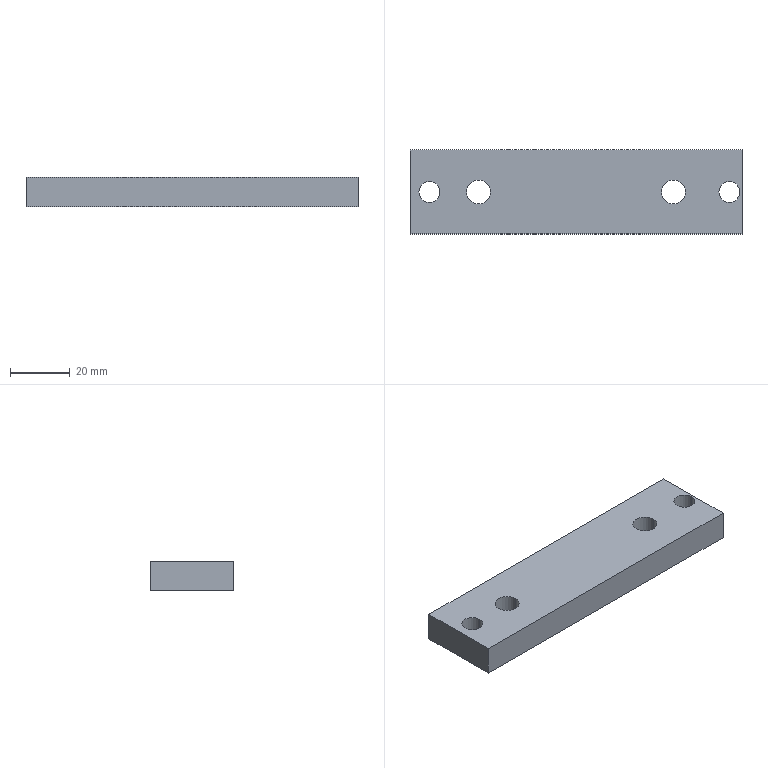Part | STEP file | 导柱Plate-2 | 1 solid | 14 faces | box 110.709 x 28 x 10 mm | volume 29224 mm3 | cylinder 8 | plane 6 | commonest cylinder face diameters 7 x4 8 x4
STEP:
#1=CARTESIAN_POINT('',(13.5,0.,10.));
#2=VERTEX_POINT('',#1);
#3=CARTESIAN_POINT('',(21.5,0.,10.));
#4=VERTEX_POINT('',#3);
#5=CARTESIAN_POINT('',(17.5,0.,10.));
#6=DIRECTION('',(0.,0.,1.));
#7=DIRECTION('',(1.,0.,0.));
#8=AXIS2_PLACEMENT_3D('',#5,#6,#7);
#9=CIRCLE('',#8,4.);
#10=EDGE_CURVE('',#2,#4,#9,.T.);
#11=ORIENTED_EDGE('',*,*,#10,.T.);
#12=CARTESIAN_POINT('',(21.5,0.,0.));
#13=VERTEX_POINT('',#12);
#14=CARTESIAN_POINT('',(21.5,0.,10.));
#15=DIRECTION('',(0.,0.,-1.));
#16=VECTOR('',#15,1000.);
#17=LINE('',#14,#16);
#18=EDGE_CURVE('',#4,#13,#17,.T.);
#19=ORIENTED_EDGE('',*,*,#18,.T.);
#20=CARTESIAN_POINT('',(13.5,0.,0.));
#21=VERTEX_POINT('',#20);
#22=CARTESIAN_POINT('',(17.5,0.,0.));
#23=DIRECTION('',(0.,0.,1.));
#24=DIRECTION('',(1.,0.,0.));
#25=AXIS2_PLACEMENT_3D('',#22,#23,#24);
#26=CIRCLE('',#25,4.);
#27=EDGE_CURVE('',#21,#13,#26,.T.);
#28=ORIENTED_EDGE('',*,*,#27,.F.);
#29=CARTESIAN_POINT('',(13.5,0.,10.));
#30=DIRECTION('',(0.,0.,-1.));
#31=VECTOR('',#30,1000.);
#32=LINE('',#29,#31);
#33=EDGE_CURVE('',#2,#21,#32,.T.);
#34=ORIENTED_EDGE('',*,*,#33,.F.);
#35=EDGE_LOOP('',(#11,#19,#28,#34));
#36=FACE_OUTER_BOUND('',#35,.T.);
#37=CARTESIAN_POINT('',(17.5,0.,10.));
#38=DIRECTION('',(0.,0.,-1.));
#39=DIRECTION('',(-1.,0.,0.));
#40=AXIS2_PLACEMENT_3D('',#37,#38,#39);
#41=CYLINDRICAL_SURFACE('',#40,4.);
#42=ADVANCED_FACE('',(#36),#41,.F.);
#43=CARTESIAN_POINT('',(78.5,0.,10.));
#44=VERTEX_POINT('',#43);
#45=CARTESIAN_POINT('',(86.5,0.,10.));
#46=VERTEX_POINT('',#45);
#47=CARTESIAN_POINT('',(82.5,0.,10.));
#48=DIRECTION('',(0.,0.,1.));
#49=DIRECTION('',(1.,0.,0.));
#50=AXIS2_PLACEMENT_3D('',#47,#48,#49);
#51=CIRCLE('',#50,4.);
#52=EDGE_CURVE('',#44,#46,#51,.T.);
#53=ORIENTED_EDGE('',*,*,#52,.T.);
#54=CARTESIAN_POINT('',(86.5,0.,0.));
#55=VERTEX_POINT('',#54);
#56=CARTESIAN_POINT('',(86.5,0.,10.));
#57=DIRECTION('',(0.,0.,-1.));
#58=VECTOR('',#57,1000.);
#59=LINE('',#56,#58);
#60=EDGE_CURVE('',#46,#55,#59,.T.);
#61=ORIENTED_EDGE('',*,*,#60,.T.);
#62=CARTESIAN_POINT('',(78.5,0.,0.));
#63=VERTEX_POINT('',#62);
#64=CARTESIAN_POINT('',(82.5,0.,0.));
#65=DIRECTION('',(0.,0.,1.));
#66=DIRECTION('',(1.,0.,0.));
#67=AXIS2_PLACEMENT_3D('',#64,#65,#66);
#68=CIRCLE('',#67,4.);
#69=EDGE_CURVE('',#63,#55,#68,.T.);
#70=ORIENTED_EDGE('',*,*,#69,.F.);
#71=CARTESIAN_POINT('',(78.5,0.,10.));
#72=DIRECTION('',(0.,0.,-1.));
#73=VECTOR('',#72,1000.);
#74=LINE('',#71,#73);
#75=EDGE_CURVE('',#44,#63,#74,.T.);
#76=ORIENTED_EDGE('',*,*,#75,.F.);
#77=EDGE_LOOP('',(#53,#61,#70,#76));
#78=FACE_OUTER_BOUND('',#77,.T.);
#79=CARTESIAN_POINT('',(82.5,0.,10.));
#80=DIRECTION('',(0.,0.,-1.));
#81=DIRECTION('',(-1.,0.,0.));
#82=AXIS2_PLACEMENT_3D('',#79,#80,#81);
#83=CYLINDRICAL_SURFACE('',#82,4.);
#84=ADVANCED_FACE('',(#78),#83,.F.);
#85=CARTESIAN_POINT('',(97.645,0.,10.));
#86=VERTEX_POINT('',#85);
#87=CARTESIAN_POINT('',(104.645,0.,10.));
#88=VERTEX_POINT('',#87);
#89=CARTESIAN_POINT('',(101.145,0.,10.));
#90=DIRECTION('',(0.,0.,1.));
#91=DIRECTION('',(1.,0.,0.));
#92=AXIS2_PLACEMENT_3D('',#89,#90,#91);
#93=CIRCLE('',#92,3.5);
#94=EDGE_CURVE('',#86,#88,#93,.T.);
#95=ORIENTED_EDGE('',*,*,#94,.T.);
#96=CARTESIAN_POINT('',(104.645,0.,0.));
#97=VERTEX_POINT('',#96);
#98=CARTESIAN_POINT('',(104.645,0.,10.));
#99=DIRECTION('',(0.,0.,-1.));
#100=VECTOR('',#99,1000.);
#101=LINE('',#98,#100);
#102=EDGE_CURVE('',#88,#97,#101,.T.);
#103=ORIENTED_EDGE('',*,*,#102,.T.);
#104=CARTESIAN_POINT('',(97.645,0.,0.));
#105=VERTEX_POINT('',#104);
#106=CARTESIAN_POINT('',(101.145,0.,0.));
#107=DIRECTION('',(0.,0.,1.));
#108=DIRECTION('',(1.,0.,0.));
#109=AXIS2_PLACEMENT_3D('',#106,#107,#108);
#110=CIRCLE('',#109,3.5);
#111=EDGE_CURVE('',#105,#97,#110,.T.);
#112=ORIENTED_EDGE('',*,*,#111,.F.);
#113=CARTESIAN_POINT('',(97.645,0.,10.));
#114=DIRECTION('',(0.,0.,-1.));
#115=VECTOR('',#114,1000.);
#116=LINE('',#113,#115);
#117=EDGE_CURVE('',#86,#105,#116,.T.);
#118=ORIENTED_EDGE('',*,*,#117,.F.);
#119=EDGE_LOOP('',(#95,#103,#112,#118));
#120=FACE_OUTER_BOUND('',#119,.T.);
#121=CARTESIAN_POINT('',(101.145,0.,10.));
#122=DIRECTION('',(0.,0.,-1.));
#123=DIRECTION('',(-1.,0.,0.));
#124=AXIS2_PLACEMENT_3D('',#121,#122,#123);
#125=CYLINDRICAL_SURFACE('',#124,3.5);
#126=ADVANCED_FACE('',(#120),#125,.F.);
#127=CARTESIAN_POINT('',(-2.355,0.,10.));
#128=VERTEX_POINT('',#127);
#129=CARTESIAN_POINT('',(4.645,0.,10.));
#130=VERTEX_POINT('',#129);
#131=CARTESIAN_POINT('',(1.145,0.,10.));
#132=DIRECTION('',(0.,0.,1.));
#133=DIRECTION('',(1.,0.,0.));
#134=AXIS2_PLACEMENT_3D('',#131,#132,#133);
#135=CIRCLE('',#134,3.5);
#136=EDGE_CURVE('',#128,#130,#135,.T.);
#137=ORIENTED_EDGE('',*,*,#136,.T.);
#138=CARTESIAN_POINT('',(4.645,0.,0.));
#139=VERTEX_POINT('',#138);
#140=CARTESIAN_POINT('',(4.645,0.,10.));
#141=DIRECTION('',(0.,0.,-1.));
#142=VECTOR('',#141,1000.);
#143=LINE('',#140,#142);
#144=EDGE_CURVE('',#130,#139,#143,.T.);
#145=ORIENTED_EDGE('',*,*,#144,.T.);
#146=CARTESIAN_POINT('',(-2.355,0.,0.));
#147=VERTEX_POINT('',#146);
#148=CARTESIAN_POINT('',(1.145,0.,0.));
#149=DIRECTION('',(0.,0.,1.));
#150=DIRECTION('',(1.,0.,0.));
#151=AXIS2_PLACEMENT_3D('',#148,#149,#150);
#152=CIRCLE('',#151,3.5);
#153=EDGE_CURVE('',#147,#139,#152,.T.);
#154=ORIENTED_EDGE('',*,*,#153,.F.);
#155=CARTESIAN_POINT('',(-2.355,0.,10.));
#156=DIRECTION('',(0.,0.,-1.));
#157=VECTOR('',#156,1000.);
#158=LINE('',#155,#157);
#159=EDGE_CURVE('',#128,#147,#158,.T.);
#160=ORIENTED_EDGE('',*,*,#159,.F.);
#161=EDGE_LOOP('',(#137,#145,#154,#160));
#162=FACE_OUTER_BOUND('',#161,.T.);
#163=CARTESIAN_POINT('',(1.145,0.,10.));
#164=DIRECTION('',(0.,0.,-1.));
#165=DIRECTION('',(-1.,0.,0.));
#166=AXIS2_PLACEMENT_3D('',#163,#164,#165);
#167=CYLINDRICAL_SURFACE('',#166,3.5);
#168=ADVANCED_FACE('',(#162),#167,.F.);
#169=ORIENTED_EDGE('',*,*,#52,.F.);
#170=CARTESIAN_POINT('',(82.5,0.,10.));
#171=DIRECTION('',(0.,0.,1.));
#172=DIRECTION('',(1.,0.,0.));
#173=AXIS2_PLACEMENT_3D('',#170,#171,#172);
#174=CIRCLE('',#173,4.);
#175=EDGE_CURVE('',#46,#44,#174,.T.);
#176=ORIENTED_EDGE('',*,*,#175,.F.);
#177=EDGE_LOOP('',(#169,#176));
#178=FACE_BOUND('',#177,.T.);
#179=ORIENTED_EDGE('',*,*,#136,.F.);
#180=CARTESIAN_POINT('',(1.145,0.,10.));
#181=DIRECTION('',(0.,0.,1.));
#182=DIRECTION('',(1.,0.,0.));
#183=AXIS2_PLACEMENT_3D('',#180,#181,#182);
#184=CIRCLE('',#183,3.5);
#185=EDGE_CURVE('',#130,#128,#184,.T.);
#186=ORIENTED_EDGE('',*,*,#185,.F.);
#187=EDGE_LOOP('',(#179,#186));
#188=FACE_BOUND('',#187,.T.);
#189=CARTESIAN_POINT('',(105.355,-14.,10.));
#190=VERTEX_POINT('',#189);
#191=CARTESIAN_POINT('',(105.355,14.,10.));
#192=VERTEX_POINT('',#191);
#193=CARTESIAN_POINT('',(105.355,-14.,10.));
#194=DIRECTION('',(0.,1.,0.));
#195=VECTOR('',#194,1000.);
#196=LINE('',#193,#195);
#197=EDGE_CURVE('',#190,#192,#196,.T.);
#198=ORIENTED_EDGE('',*,*,#197,.T.);
#199=CARTESIAN_POINT('',(-5.355,14.,10.));
#200=VERTEX_POINT('',#199);
#201=CARTESIAN_POINT('',(-5.355,14.,10.));
#202=DIRECTION('',(-1.,0.,0.));
#203=VECTOR('',#202,1000.);
#204=LINE('',#201,#203);
#205=EDGE_CURVE('',#192,#200,#204,.T.);
#206=ORIENTED_EDGE('',*,*,#205,.T.);
#207=CARTESIAN_POINT('',(-5.355,-14.,10.));
#208=VERTEX_POINT('',#207);
#209=CARTESIAN_POINT('',(-5.355,-14.,10.));
#210=DIRECTION('',(0.,-1.,0.));
#211=VECTOR('',#210,1000.);
#212=LINE('',#209,#211);
#213=EDGE_CURVE('',#200,#208,#212,.T.);
#214=ORIENTED_EDGE('',*,*,#213,.T.);
#215=CARTESIAN_POINT('',(-5.355,-14.,10.));
#216=DIRECTION('',(1.,0.,0.));
#217=VECTOR('',#216,1000.);
#218=LINE('',#215,#217);
#219=EDGE_CURVE('',#208,#190,#218,.T.);
#220=ORIENTED_EDGE('',*,*,#219,.T.);
#221=EDGE_LOOP('',(#198,#206,#214,#220));
#222=FACE_OUTER_BOUND('',#221,.T.);
#223=ORIENTED_EDGE('',*,*,#94,.F.);
#224=CARTESIAN_POINT('',(101.145,0.,10.));
#225=DIRECTION('',(0.,0.,1.));
#226=DIRECTION('',(1.,0.,0.));
#227=AXIS2_PLACEMENT_3D('',#224,#225,#226);
#228=CIRCLE('',#227,3.5);
#229=EDGE_CURVE('',#88,#86,#228,.T.);
#230=ORIENTED_EDGE('',*,*,#229,.F.);
#231=EDGE_LOOP('',(#223,#230));
#232=FACE_BOUND('',#231,.T.);
#233=ORIENTED_EDGE('',*,*,#10,.F.);
#234=CARTESIAN_POINT('',(17.5,0.,10.));
#235=DIRECTION('',(0.,0.,1.));
#236=DIRECTION('',(1.,0.,0.));
#237=AXIS2_PLACEMENT_3D('',#234,#235,#236);
#238=CIRCLE('',#237,4.);
#239=EDGE_CURVE('',#4,#2,#238,.T.);
#240=ORIENTED_EDGE('',*,*,#239,.F.);
#241=EDGE_LOOP('',(#233,#240));
#242=FACE_BOUND('',#241,.T.);
#243=CARTESIAN_POINT('',(105.355,14.,10.));
#244=DIRECTION('',(0.,0.,-1.));
#245=DIRECTION('',(-1.,0.,0.));
#246=AXIS2_PLACEMENT_3D('',#243,#244,#245);
#247=PLANE('',#246);
#248=ADVANCED_FACE('',(#178,#188,#222,#232,#242),#247,.F.);
#249=ORIENTED_EDGE('',*,*,#69,.T.);
#250=CARTESIAN_POINT('',(82.5,0.,0.));
#251=DIRECTION('',(0.,0.,1.));
#252=DIRECTION('',(1.,0.,0.));
#253=AXIS2_PLACEMENT_3D('',#250,#251,#252);
#254=CIRCLE('',#253,4.);
#255=EDGE_CURVE('',#55,#63,#254,.T.);
#256=ORIENTED_EDGE('',*,*,#255,.T.);
#257=EDGE_LOOP('',(#249,#256));
#258=FACE_BOUND('',#257,.T.);
#259=ORIENTED_EDGE('',*,*,#153,.T.);
#260=CARTESIAN_POINT('',(1.145,0.,0.));
#261=DIRECTION('',(0.,0.,1.));
#262=DIRECTION('',(1.,0.,0.));
#263=AXIS2_PLACEMENT_3D('',#260,#261,#262);
#264=CIRCLE('',#263,3.5);
#265=EDGE_CURVE('',#139,#147,#264,.T.);
#266=ORIENTED_EDGE('',*,*,#265,.T.);
#267=EDGE_LOOP('',(#259,#266));
#268=FACE_BOUND('',#267,.T.);
#269=CARTESIAN_POINT('',(105.355,-14.,0.));
#270=VERTEX_POINT('',#269);
#271=CARTESIAN_POINT('',(105.355,14.,0.));
#272=VERTEX_POINT('',#271);
#273=CARTESIAN_POINT('',(105.355,-14.,0.));
#274=DIRECTION('',(0.,1.,0.));
#275=VECTOR('',#274,1000.);
#276=LINE('',#273,#275);
#277=EDGE_CURVE('',#270,#272,#276,.T.);
#278=ORIENTED_EDGE('',*,*,#277,.F.);
#279=CARTESIAN_POINT('',(-5.355,-14.,0.));
#280=VERTEX_POINT('',#279);
#281=CARTESIAN_POINT('',(-5.355,-14.,0.));
#282=DIRECTION('',(1.,0.,0.));
#283=VECTOR('',#282,1000.);
#284=LINE('',#281,#283);
#285=EDGE_CURVE('',#280,#270,#284,.T.);
#286=ORIENTED_EDGE('',*,*,#285,.F.);
#287=CARTESIAN_POINT('',(-5.355,14.,0.));
#288=VERTEX_POINT('',#287);
#289=CARTESIAN_POINT('',(-5.355,-14.,0.));
#290=DIRECTION('',(0.,-1.,0.));
#291=VECTOR('',#290,1000.);
#292=LINE('',#289,#291);
#293=EDGE_CURVE('',#288,#280,#292,.T.);
#294=ORIENTED_EDGE('',*,*,#293,.F.);
#295=CARTESIAN_POINT('',(-5.355,14.,0.));
#296=DIRECTION('',(-1.,0.,0.));
#297=VECTOR('',#296,1000.);
#298=LINE('',#295,#297);
#299=EDGE_CURVE('',#272,#288,#298,.T.);
#300=ORIENTED_EDGE('',*,*,#299,.F.);
#301=EDGE_LOOP('',(#278,#286,#294,#300));
#302=FACE_OUTER_BOUND('',#301,.T.);
#303=ORIENTED_EDGE('',*,*,#111,.T.);
#304=CARTESIAN_POINT('',(101.145,0.,0.));
#305=DIRECTION('',(0.,0.,1.));
#306=DIRECTION('',(1.,0.,0.));
#307=AXIS2_PLACEMENT_3D('',#304,#305,#306);
#308=CIRCLE('',#307,3.5);
#309=EDGE_CURVE('',#97,#105,#308,.T.);
#310=ORIENTED_EDGE('',*,*,#309,.T.);
#311=EDGE_LOOP('',(#303,#310));
#312=FACE_BOUND('',#311,.T.);
#313=ORIENTED_EDGE('',*,*,#27,.T.);
#314=CARTESIAN_POINT('',(17.5,0.,0.));
#315=DIRECTION('',(0.,0.,1.));
#316=DIRECTION('',(1.,0.,0.));
#317=AXIS2_PLACEMENT_3D('',#314,#315,#316);
#318=CIRCLE('',#317,4.);
#319=EDGE_CURVE('',#13,#21,#318,.T.);
#320=ORIENTED_EDGE('',*,*,#319,.T.);
#321=EDGE_LOOP('',(#313,#320));
#322=FACE_BOUND('',#321,.T.);
#323=CARTESIAN_POINT('',(105.355,14.,0.));
#324=DIRECTION('',(0.,0.,-1.));
#325=DIRECTION('',(-1.,0.,0.));
#326=AXIS2_PLACEMENT_3D('',#323,#324,#325);
#327=PLANE('',#326);
#328=ADVANCED_FACE('',(#258,#268,#302,#312,#322),#327,.T.);
#329=ORIENTED_EDGE('',*,*,#277,.T.);
#330=CARTESIAN_POINT('',(105.355,14.,10.));
#331=DIRECTION('',(0.,0.,-1.));
#332=VECTOR('',#331,1000.);
#333=LINE('',#330,#332);
#334=EDGE_CURVE('',#192,#272,#333,.T.);
#335=ORIENTED_EDGE('',*,*,#334,.F.);
#336=ORIENTED_EDGE('',*,*,#197,.F.);
#337=CARTESIAN_POINT('',(105.355,-14.,10.));
#338=DIRECTION('',(0.,0.,-1.));
#339=VECTOR('',#338,1000.);
#340=LINE('',#337,#339);
#341=EDGE_CURVE('',#190,#270,#340,.T.);
#342=ORIENTED_EDGE('',*,*,#341,.T.);
#343=EDGE_LOOP('',(#329,#335,#336,#342));
#344=FACE_OUTER_BOUND('',#343,.T.);
#345=CARTESIAN_POINT('',(105.355,-14.,10.));
#346=DIRECTION('',(-1.,0.,0.));
#347=DIRECTION('',(0.,0.,1.));
#348=AXIS2_PLACEMENT_3D('',#345,#346,#347);
#349=PLANE('',#348);
#350=ADVANCED_FACE('',(#344),#349,.F.);
#351=ORIENTED_EDGE('',*,*,#299,.T.);
#352=CARTESIAN_POINT('',(-5.355,14.,10.));
#353=DIRECTION('',(0.,0.,-1.));
#354=VECTOR('',#353,1000.);
#355=LINE('',#352,#354);
#356=EDGE_CURVE('',#200,#288,#355,.T.);
#357=ORIENTED_EDGE('',*,*,#356,.F.);
#358=ORIENTED_EDGE('',*,*,#205,.F.);
#359=ORIENTED_EDGE('',*,*,#334,.T.);
#360=EDGE_LOOP('',(#351,#357,#358,#359));
#361=FACE_OUTER_BOUND('',#360,.T.);
#362=CARTESIAN_POINT('',(-5.355,14.,10.));
#363=DIRECTION('',(0.,-1.,0.));
#364=DIRECTION('',(0.,0.,-1.));
#365=AXIS2_PLACEMENT_3D('',#362,#363,#364);
#366=PLANE('',#365);
#367=ADVANCED_FACE('',(#361),#366,.F.);
#368=ORIENTED_EDGE('',*,*,#293,.T.);
#369=CARTESIAN_POINT('',(-5.355,-14.,10.));
#370=DIRECTION('',(0.,0.,-1.));
#371=VECTOR('',#370,1000.);
#372=LINE('',#369,#371);
#373=EDGE_CURVE('',#208,#280,#372,.T.);
#374=ORIENTED_EDGE('',*,*,#373,.F.);
#375=ORIENTED_EDGE('',*,*,#213,.F.);
#376=ORIENTED_EDGE('',*,*,#356,.T.);
#377=EDGE_LOOP('',(#368,#374,#375,#376));
#378=FACE_OUTER_BOUND('',#377,.T.);
#379=CARTESIAN_POINT('',(-5.355,-14.,10.));
#380=DIRECTION('',(1.,0.,0.));
#381=DIRECTION('',(0.,0.,-1.));
#382=AXIS2_PLACEMENT_3D('',#379,#380,#381);
#383=PLANE('',#382);
#384=ADVANCED_FACE('',(#378),#383,.F.);
#385=ORIENTED_EDGE('',*,*,#285,.T.);
#386=ORIENTED_EDGE('',*,*,#341,.F.);
#387=ORIENTED_EDGE('',*,*,#219,.F.);
#388=ORIENTED_EDGE('',*,*,#373,.T.);
#389=EDGE_LOOP('',(#385,#386,#387,#388));
#390=FACE_OUTER_BOUND('',#389,.T.);
#391=CARTESIAN_POINT('',(-5.355,-14.,10.));
#392=DIRECTION('',(0.,1.,0.));
#393=DIRECTION('',(0.,0.,1.));
#394=AXIS2_PLACEMENT_3D('',#391,#392,#393);
#395=PLANE('',#394);
#396=ADVANCED_FACE('',(#390),#395,.F.);
#397=ORIENTED_EDGE('',*,*,#144,.F.);
#398=ORIENTED_EDGE('',*,*,#185,.T.);
#399=ORIENTED_EDGE('',*,*,#159,.T.);
#400=ORIENTED_EDGE('',*,*,#265,.F.);
#401=EDGE_LOOP('',(#397,#398,#399,#400));
#402=FACE_OUTER_BOUND('',#401,.T.);
#403=CARTESIAN_POINT('',(1.145,0.,10.));
#404=DIRECTION('',(0.,0.,-1.));
#405=DIRECTION('',(-1.,0.,0.));
#406=AXIS2_PLACEMENT_3D('',#403,#404,#405);
#407=CYLINDRICAL_SURFACE('',#406,3.5);
#408=ADVANCED_FACE('',(#402),#407,.F.);
#409=ORIENTED_EDGE('',*,*,#102,.F.);
#410=ORIENTED_EDGE('',*,*,#229,.T.);
#411=ORIENTED_EDGE('',*,*,#117,.T.);
#412=ORIENTED_EDGE('',*,*,#309,.F.);
#413=EDGE_LOOP('',(#409,#410,#411,#412));
#414=FACE_OUTER_BOUND('',#413,.T.);
#415=CARTESIAN_POINT('',(101.145,0.,10.));
#416=DIRECTION('',(0.,0.,-1.));
#417=DIRECTION('',(-1.,0.,0.));
#418=AXIS2_PLACEMENT_3D('',#415,#416,#417);
#419=CYLINDRICAL_SURFACE('',#418,3.5);
#420=ADVANCED_FACE('',(#414),#419,.F.);
#421=ORIENTED_EDGE('',*,*,#60,.F.);
#422=ORIENTED_EDGE('',*,*,#175,.T.);
#423=ORIENTED_EDGE('',*,*,#75,.T.);
#424=ORIENTED_EDGE('',*,*,#255,.F.);
#425=EDGE_LOOP('',(#421,#422,#423,#424));
#426=FACE_OUTER_BOUND('',#425,.T.);
#427=CARTESIAN_POINT('',(82.5,0.,10.));
#428=DIRECTION('',(0.,0.,-1.));
#429=DIRECTION('',(-1.,0.,0.));
#430=AXIS2_PLACEMENT_3D('',#427,#428,#429);
#431=CYLINDRICAL_SURFACE('',#430,4.);
#432=ADVANCED_FACE('',(#426),#431,.F.);
#433=ORIENTED_EDGE('',*,*,#18,.F.);
#434=ORIENTED_EDGE('',*,*,#239,.T.);
#435=ORIENTED_EDGE('',*,*,#33,.T.);
#436=ORIENTED_EDGE('',*,*,#319,.F.);
#437=EDGE_LOOP('',(#433,#434,#435,#436));
#438=FACE_OUTER_BOUND('',#437,.T.);
#439=CARTESIAN_POINT('',(17.5,0.,10.));
#440=DIRECTION('',(0.,0.,-1.));
#441=DIRECTION('',(-1.,0.,0.));
#442=AXIS2_PLACEMENT_3D('',#439,#440,#441);
#443=CYLINDRICAL_SURFACE('',#442,4.);
#444=ADVANCED_FACE('',(#438),#443,.F.);
#445=CLOSED_SHELL('',(#42,#84,#126,#168,#248,#328,#350,#367,#384,#396,#408,#420,#432,#444));
#446=MANIFOLD_SOLID_BREP('',#445);
#447=CARTESIAN_POINT('',(0.,0.,0.));
#448=DIRECTION('',(0.,0.,1.));
#449=DIRECTION('',(1.,0.,0.));
#450=AXIS2_PLACEMENT_3D('',#447,#448,#449);
#451=(LENGTH_UNIT()NAMED_UNIT(*)SI_UNIT(.MILLI.,.METRE.));
#452=UNCERTAINTY_MEASURE_WITH_UNIT(LENGTH_MEASURE(0.00001),#451,'','');
#453=(NAMED_UNIT(*)PLANE_ANGLE_UNIT()SI_UNIT($,.RADIAN.));
#454=(NAMED_UNIT(*)SI_UNIT($,.STERADIAN.)SOLID_ANGLE_UNIT());
#455=(GEOMETRIC_REPRESENTATION_CONTEXT(3)GLOBAL_UNCERTAINTY_ASSIGNED_CONTEXT((#452))GLOBAL_UNIT_ASSIGNED_CONTEXT((#451,#453,#454))REPRESENTATION_CONTEXT('',''));
#456=ADVANCED_BREP_SHAPE_REPRESENTATION('',(#446,#450),#455);